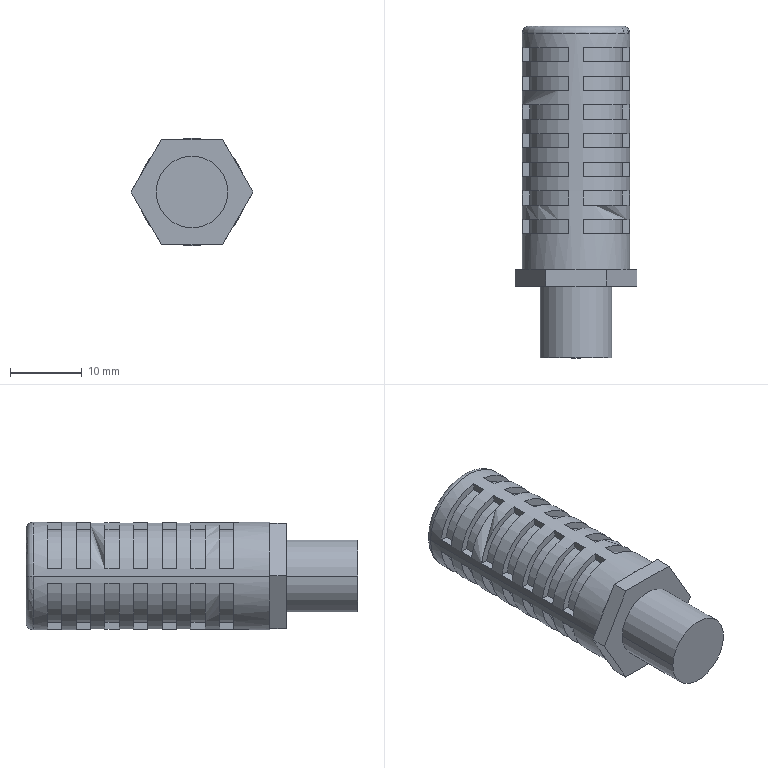Part | STEP file | 1 solid | 176 faces | box 17 x 46.3 x 15 mm | volume 6244 mm3 | plane 136 | cylinder 36 | torus 2 | cone 2 | commonest cylinder face diameters 13 x28 3 x2 5 x2 10 x2 15 x2